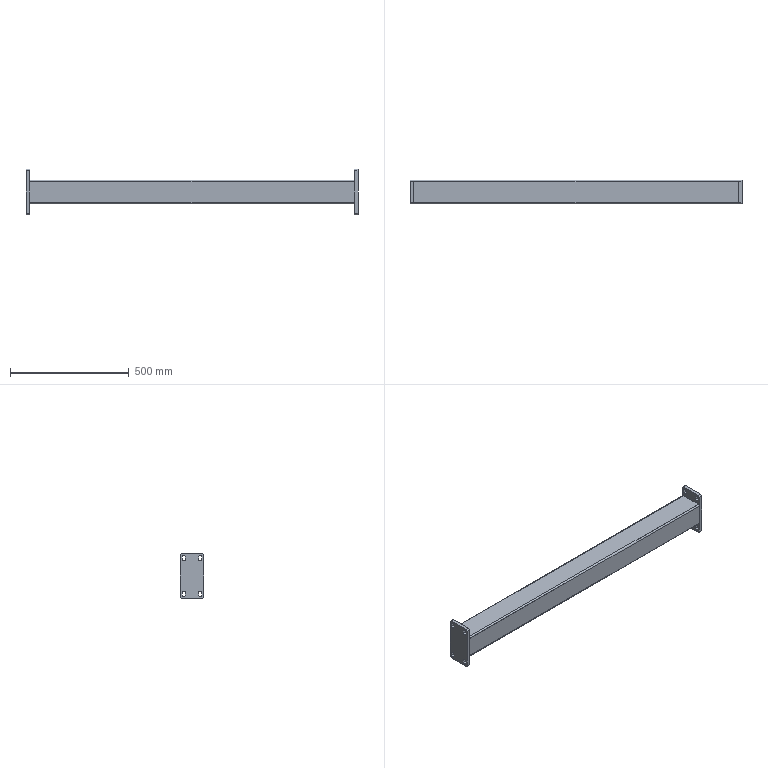Part | SolidWorks | features HoleWzd 1, ICE 1, MirrorSolid 1, WeldMemberFeat 1, WeldmentFeature 1 | 3 solids | 78 faces | box 1395 x 100 x 190 mm | volume 2190418 mm3 | plane 46 | cylinder 32 | commonest cylinder face diameters 13.5 x24 6.4 x4 12.8 x4